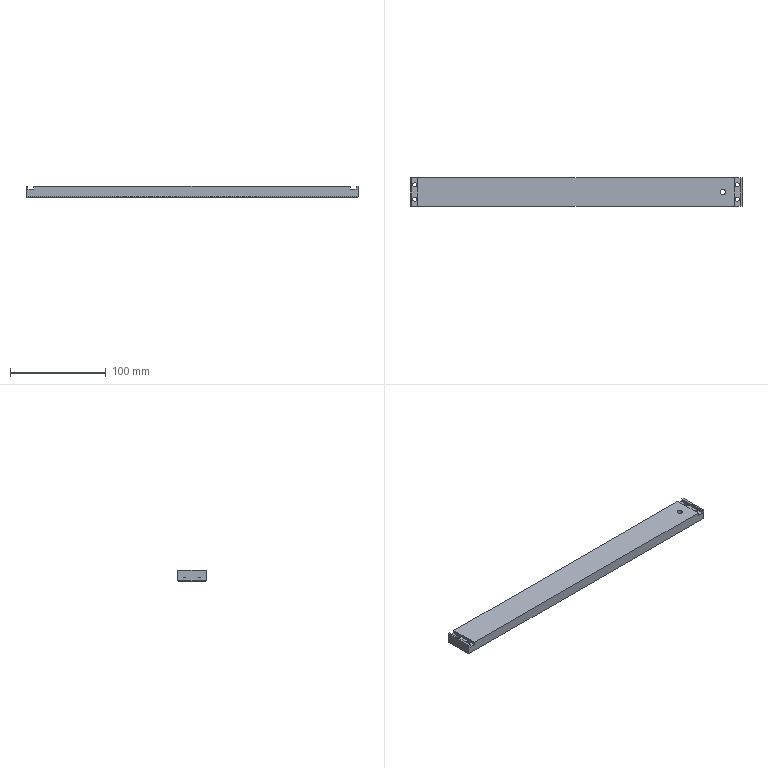Part | NX | 1 solid | 32 faces | box 346 x 30 x 11.5 mm | volume 116609 mm3 | plane 22 | cylinder 9 | cone 1 | commonest cylinder face diameters 4.5 x4 8 x4 5.5 x1
STEP:
#1=CARTESIAN_POINT('',(0.,30.,0.75));
#2=VERTEX_POINT('',#1);
#3=CARTESIAN_POINT('',(0.75,29.25,0.));
#4=VERTEX_POINT('',#3);
#5=CARTESIAN_POINT('',(0.,30.,0.75));
#6=DIRECTION('',(0.5774,-0.5774,-0.5774));
#7=VECTOR('',#6,1000.);
#8=LINE('',#5,#7);
#9=EDGE_CURVE('',#2,#4,#8,.T.);
#10=ORIENTED_EDGE('',*,*,#9,.T.);
#11=CARTESIAN_POINT('',(0.75,0.75,0.));
#12=VERTEX_POINT('',#11);
#13=CARTESIAN_POINT('',(0.75,30.,0.));
#14=DIRECTION('',(0.,1.,0.));
#15=VECTOR('',#14,1000.);
#16=LINE('',#13,#15);
#17=EDGE_CURVE('',#12,#4,#16,.T.);
#18=ORIENTED_EDGE('',*,*,#17,.F.);
#19=CARTESIAN_POINT('',(0.,0.,0.75));
#20=VERTEX_POINT('',#19);
#21=CARTESIAN_POINT('',(0.,0.,0.75));
#22=DIRECTION('',(-0.5774,-0.5774,0.5774));
#23=VECTOR('',#22,1000.);
#24=LINE('',#21,#23);
#25=EDGE_CURVE('',#12,#20,#24,.T.);
#26=ORIENTED_EDGE('',*,*,#25,.T.);
#27=CARTESIAN_POINT('',(0.,0.,0.75));
#28=DIRECTION('',(0.,-1.,0.));
#29=VECTOR('',#28,1000.);
#30=LINE('',#27,#29);
#31=EDGE_CURVE('',#2,#20,#30,.T.);
#32=ORIENTED_EDGE('',*,*,#31,.F.);
#33=EDGE_LOOP('',(#10,#18,#26,#32));
#34=FACE_BOUND('',#33,.T.);
#35=CARTESIAN_POINT('',(0.,0.,0.75));
#36=DIRECTION('',(-0.7071,0.,-0.7071));
#37=DIRECTION('',(0.,1.,0.));
#38=AXIS2_PLACEMENT_3D('',#35,#36,#37);
#39=PLANE('',#38);
#40=ADVANCED_FACE('',(#34),#39,.T.);
#41=CARTESIAN_POINT('',(345.25,0.75,0.));
#42=VERTEX_POINT('',#41);
#43=CARTESIAN_POINT('',(346.,0.,0.75));
#44=VERTEX_POINT('',#43);
#45=CARTESIAN_POINT('',(230.667,115.333,-114.583));
#46=DIRECTION('',(0.5774,-0.5774,0.5774));
#47=VECTOR('',#46,1000.);
#48=LINE('',#45,#47);
#49=EDGE_CURVE('',#42,#44,#48,.T.);
#50=ORIENTED_EDGE('',*,*,#49,.T.);
#51=CARTESIAN_POINT('',(346.,0.,0.75));
#52=DIRECTION('',(1.,0.,0.));
#53=VECTOR('',#52,1000.);
#54=LINE('',#51,#53);
#55=EDGE_CURVE('',#20,#44,#54,.T.);
#56=ORIENTED_EDGE('',*,*,#55,.F.);
#57=ORIENTED_EDGE('',*,*,#25,.F.);
#58=CARTESIAN_POINT('',(0.,0.75,0.));
#59=DIRECTION('',(-1.,0.,0.));
#60=VECTOR('',#59,1000.);
#61=LINE('',#58,#60);
#62=EDGE_CURVE('',#42,#12,#61,.T.);
#63=ORIENTED_EDGE('',*,*,#62,.F.);
#64=EDGE_LOOP('',(#50,#56,#57,#63));
#65=FACE_BOUND('',#64,.T.);
#66=CARTESIAN_POINT('',(0.,0.,0.75));
#67=DIRECTION('',(0.,-0.7071,-0.7071));
#68=DIRECTION('',(-1.,0.,0.));
#69=AXIS2_PLACEMENT_3D('',#66,#67,#68);
#70=PLANE('',#69);
#71=ADVANCED_FACE('',(#65),#70,.T.);
#72=CARTESIAN_POINT('',(346.,30.,0.75));
#73=VERTEX_POINT('',#72);
#74=CARTESIAN_POINT('',(345.25,29.25,0.));
#75=VERTEX_POINT('',#74);
#76=CARTESIAN_POINT('',(336.,20.,-9.25));
#77=DIRECTION('',(-0.5774,-0.5774,-0.5774));
#78=VECTOR('',#77,1000.);
#79=LINE('',#76,#78);
#80=EDGE_CURVE('',#73,#75,#79,.T.);
#81=ORIENTED_EDGE('',*,*,#80,.T.);
#82=CARTESIAN_POINT('',(346.,29.25,0.));
#83=DIRECTION('',(1.,0.,0.));
#84=VECTOR('',#83,1000.);
#85=LINE('',#82,#84);
#86=EDGE_CURVE('',#4,#75,#85,.T.);
#87=ORIENTED_EDGE('',*,*,#86,.F.);
#88=ORIENTED_EDGE('',*,*,#9,.F.);
#89=CARTESIAN_POINT('',(0.,30.,0.75));
#90=DIRECTION('',(-1.,0.,0.));
#91=VECTOR('',#90,1000.);
#92=LINE('',#89,#91);
#93=EDGE_CURVE('',#73,#2,#92,.T.);
#94=ORIENTED_EDGE('',*,*,#93,.F.);
#95=EDGE_LOOP('',(#81,#87,#88,#94));
#96=FACE_BOUND('',#95,.T.);
#97=CARTESIAN_POINT('',(0.,30.,0.75));
#98=DIRECTION('',(0.,0.7071,-0.7071));
#99=DIRECTION('',(1.,0.,0.));
#100=AXIS2_PLACEMENT_3D('',#97,#98,#99);
#101=PLANE('',#100);
#102=ADVANCED_FACE('',(#96),#101,.T.);
#103=ORIENTED_EDGE('',*,*,#49,.F.);
#104=CARTESIAN_POINT('',(345.25,0.,0.));
#105=DIRECTION('',(0.,-1.,0.));
#106=VECTOR('',#105,1000.);
#107=LINE('',#104,#106);
#108=EDGE_CURVE('',#75,#42,#107,.T.);
#109=ORIENTED_EDGE('',*,*,#108,.F.);
#110=ORIENTED_EDGE('',*,*,#80,.F.);
#111=CARTESIAN_POINT('',(346.,30.,0.75));
#112=DIRECTION('',(0.,1.,0.));
#113=VECTOR('',#112,1000.);
#114=LINE('',#111,#113);
#115=EDGE_CURVE('',#44,#73,#114,.T.);
#116=ORIENTED_EDGE('',*,*,#115,.F.);
#117=EDGE_LOOP('',(#103,#109,#110,#116));
#118=FACE_BOUND('',#117,.T.);
#119=CARTESIAN_POINT('',(346.,0.,0.75));
#120=DIRECTION('',(0.7071,0.,-0.7071));
#121=DIRECTION('',(0.,-1.,0.));
#122=AXIS2_PLACEMENT_3D('',#119,#120,#121);
#123=PLANE('',#122);
#124=ADVANCED_FACE('',(#118),#123,.T.);
#125=CARTESIAN_POINT('',(1.,22.5,4.));
#126=VERTEX_POINT('',#125);
#127=CARTESIAN_POINT('',(5.,22.5,4.));
#128=DIRECTION('',(0.,0.,-1.));
#129=DIRECTION('',(-1.,0.,0.));
#130=AXIS2_PLACEMENT_3D('',#127,#128,#129);
#131=CIRCLE('',#130,4.);
#132=EDGE_CURVE('',#126,#126,#131,.T.);
#133=ORIENTED_EDGE('',*,*,#132,.T.);
#134=EDGE_LOOP('',(#133));
#135=FACE_BOUND('',#134,.T.);
#136=CARTESIAN_POINT('',(2.75,22.5,4.));
#137=VERTEX_POINT('',#136);
#138=CARTESIAN_POINT('',(5.,22.5,4.));
#139=DIRECTION('',(0.,0.,-1.));
#140=DIRECTION('',(-1.,0.,0.));
#141=AXIS2_PLACEMENT_3D('',#138,#139,#140);
#142=CIRCLE('',#141,2.25);
#143=EDGE_CURVE('',#137,#137,#142,.T.);
#144=ORIENTED_EDGE('',*,*,#143,.F.);
#145=EDGE_LOOP('',(#144));
#146=FACE_BOUND('',#145,.T.);
#147=CARTESIAN_POINT('',(7.25,22.5,4.));
#148=DIRECTION('',(0.,0.,1.));
#149=DIRECTION('',(1.,0.,0.));
#150=AXIS2_PLACEMENT_3D('',#147,#148,#149);
#151=PLANE('',#150);
#152=ADVANCED_FACE('',(#135,#146),#151,.F.);
#153=CARTESIAN_POINT('',(9.,7.5,4.));
#154=VERTEX_POINT('',#153);
#155=CARTESIAN_POINT('',(5.,7.5,4.));
#156=DIRECTION('',(0.,0.,-1.));
#157=DIRECTION('',(1.,0.,0.));
#158=AXIS2_PLACEMENT_3D('',#155,#156,#157);
#159=CIRCLE('',#158,4.);
#160=EDGE_CURVE('',#154,#154,#159,.T.);
#161=ORIENTED_EDGE('',*,*,#160,.T.);
#162=EDGE_LOOP('',(#161));
#163=FACE_BOUND('',#162,.T.);
#164=CARTESIAN_POINT('',(7.25,7.5,4.));
#165=VERTEX_POINT('',#164);
#166=CARTESIAN_POINT('',(5.,7.5,4.));
#167=DIRECTION('',(0.,0.,-1.));
#168=DIRECTION('',(1.,0.,0.));
#169=AXIS2_PLACEMENT_3D('',#166,#167,#168);
#170=CIRCLE('',#169,2.25);
#171=EDGE_CURVE('',#165,#165,#170,.T.);
#172=ORIENTED_EDGE('',*,*,#171,.F.);
#173=EDGE_LOOP('',(#172));
#174=FACE_BOUND('',#173,.T.);
#175=CARTESIAN_POINT('',(7.25,22.5,4.));
#176=DIRECTION('',(0.,0.,1.));
#177=DIRECTION('',(1.,0.,0.));
#178=AXIS2_PLACEMENT_3D('',#175,#176,#177);
#179=PLANE('',#178);
#180=ADVANCED_FACE('',(#163,#174),#179,.F.);
#181=CARTESIAN_POINT('',(8.,30.,8.5));
#182=VERTEX_POINT('',#181);
#183=CARTESIAN_POINT('',(8.,30.,11.5));
#184=VERTEX_POINT('',#183);
#185=CARTESIAN_POINT('',(8.,30.,11.5));
#186=DIRECTION('',(0.,0.,1.));
#187=VECTOR('',#186,1000.);
#188=LINE('',#185,#187);
#189=EDGE_CURVE('',#182,#184,#188,.T.);
#190=ORIENTED_EDGE('',*,*,#189,.F.);
#191=CARTESIAN_POINT('',(8.,0.,8.5));
#192=VERTEX_POINT('',#191);
#193=CARTESIAN_POINT('',(8.,0.,8.5));
#194=DIRECTION('',(0.,1.,0.));
#195=VECTOR('',#194,1000.);
#196=LINE('',#193,#195);
#197=EDGE_CURVE('',#192,#182,#196,.T.);
#198=ORIENTED_EDGE('',*,*,#197,.F.);
#199=CARTESIAN_POINT('',(8.,0.,11.5));
#200=VERTEX_POINT('',#199);
#201=CARTESIAN_POINT('',(8.,0.,11.5));
#202=DIRECTION('',(0.,0.,1.));
#203=VECTOR('',#202,1000.);
#204=LINE('',#201,#203);
#205=EDGE_CURVE('',#192,#200,#204,.T.);
#206=ORIENTED_EDGE('',*,*,#205,.T.);
#207=CARTESIAN_POINT('',(8.,0.,11.5));
#208=DIRECTION('',(0.,1.,0.));
#209=VECTOR('',#208,1000.);
#210=LINE('',#207,#209);
#211=EDGE_CURVE('',#200,#184,#210,.T.);
#212=ORIENTED_EDGE('',*,*,#211,.T.);
#213=EDGE_LOOP('',(#190,#198,#206,#212));
#214=FACE_BOUND('',#213,.T.);
#215=CARTESIAN_POINT('',(8.,0.,11.5));
#216=DIRECTION('',(-1.,0.,0.));
#217=DIRECTION('',(0.,0.,1.));
#218=AXIS2_PLACEMENT_3D('',#215,#216,#217);
#219=PLANE('',#218);
#220=ADVANCED_FACE('',(#214),#219,.T.);
#221=CARTESIAN_POINT('',(2.,30.,8.5));
#222=VERTEX_POINT('',#221);
#223=CARTESIAN_POINT('',(2.,30.,8.5));
#224=DIRECTION('',(1.,0.,0.));
#225=VECTOR('',#224,1000.);
#226=LINE('',#223,#225);
#227=EDGE_CURVE('',#222,#182,#226,.T.);
#228=ORIENTED_EDGE('',*,*,#227,.F.);
#229=CARTESIAN_POINT('',(2.,0.,8.5));
#230=VERTEX_POINT('',#229);
#231=CARTESIAN_POINT('',(2.,0.,8.5));
#232=DIRECTION('',(0.,1.,0.));
#233=VECTOR('',#232,1000.);
#234=LINE('',#231,#233);
#235=EDGE_CURVE('',#230,#222,#234,.T.);
#236=ORIENTED_EDGE('',*,*,#235,.F.);
#237=CARTESIAN_POINT('',(2.,0.,8.5));
#238=DIRECTION('',(1.,0.,0.));
#239=VECTOR('',#238,1000.);
#240=LINE('',#237,#239);
#241=EDGE_CURVE('',#230,#192,#240,.T.);
#242=ORIENTED_EDGE('',*,*,#241,.T.);
#243=ORIENTED_EDGE('',*,*,#197,.T.);
#244=EDGE_LOOP('',(#228,#236,#242,#243));
#245=FACE_BOUND('',#244,.T.);
#246=CARTESIAN_POINT('',(7.25,7.5,8.5));
#247=VERTEX_POINT('',#246);
#248=CARTESIAN_POINT('',(5.,7.5,8.5));
#249=DIRECTION('',(0.,0.,1.));
#250=DIRECTION('',(1.,0.,0.));
#251=AXIS2_PLACEMENT_3D('',#248,#249,#250);
#252=CIRCLE('',#251,2.25);
#253=EDGE_CURVE('',#247,#247,#252,.T.);
#254=ORIENTED_EDGE('',*,*,#253,.F.);
#255=EDGE_LOOP('',(#254));
#256=FACE_BOUND('',#255,.T.);
#257=CARTESIAN_POINT('',(7.25,22.5,8.5));
#258=VERTEX_POINT('',#257);
#259=CARTESIAN_POINT('',(5.,22.5,8.5));
#260=DIRECTION('',(0.,0.,1.));
#261=DIRECTION('',(1.,0.,0.));
#262=AXIS2_PLACEMENT_3D('',#259,#260,#261);
#263=CIRCLE('',#262,2.25);
#264=EDGE_CURVE('',#258,#258,#263,.T.);
#265=ORIENTED_EDGE('',*,*,#264,.F.);
#266=EDGE_LOOP('',(#265));
#267=FACE_BOUND('',#266,.T.);
#268=CARTESIAN_POINT('',(2.,0.,8.5));
#269=DIRECTION('',(0.,0.,1.));
#270=DIRECTION('',(1.,0.,0.));
#271=AXIS2_PLACEMENT_3D('',#268,#269,#270);
#272=PLANE('',#271);
#273=ADVANCED_FACE('',(#245,#256,#267),#272,.T.);
#274=CARTESIAN_POINT('',(2.,30.,11.5));
#275=VERTEX_POINT('',#274);
#276=CARTESIAN_POINT('',(2.,30.,11.5));
#277=DIRECTION('',(0.,0.,-1.));
#278=VECTOR('',#277,1000.);
#279=LINE('',#276,#278);
#280=EDGE_CURVE('',#275,#222,#279,.T.);
#281=ORIENTED_EDGE('',*,*,#280,.F.);
#282=CARTESIAN_POINT('',(2.,0.,11.5));
#283=VERTEX_POINT('',#282);
#284=CARTESIAN_POINT('',(2.,0.,11.5));
#285=DIRECTION('',(0.,1.,0.));
#286=VECTOR('',#285,1000.);
#287=LINE('',#284,#286);
#288=EDGE_CURVE('',#283,#275,#287,.T.);
#289=ORIENTED_EDGE('',*,*,#288,.F.);
#290=CARTESIAN_POINT('',(2.,0.,11.5));
#291=DIRECTION('',(0.,0.,-1.));
#292=VECTOR('',#291,1000.);
#293=LINE('',#290,#292);
#294=EDGE_CURVE('',#283,#230,#293,.T.);
#295=ORIENTED_EDGE('',*,*,#294,.T.);
#296=ORIENTED_EDGE('',*,*,#235,.T.);
#297=EDGE_LOOP('',(#281,#289,#295,#296));
#298=FACE_BOUND('',#297,.T.);
#299=CARTESIAN_POINT('',(2.,0.,11.5));
#300=DIRECTION('',(1.,0.,0.));
#301=DIRECTION('',(0.,0.,-1.));
#302=AXIS2_PLACEMENT_3D('',#299,#300,#301);
#303=PLANE('',#302);
#304=ADVANCED_FACE('',(#298),#303,.T.);
#305=CARTESIAN_POINT('',(345.,22.5,4.));
#306=VERTEX_POINT('',#305);
#307=CARTESIAN_POINT('',(341.,22.5,4.));
#308=DIRECTION('',(0.,0.,-1.));
#309=DIRECTION('',(1.,0.,0.));
#310=AXIS2_PLACEMENT_3D('',#307,#308,#309);
#311=CIRCLE('',#310,4.);
#312=EDGE_CURVE('',#306,#306,#311,.T.);
#313=ORIENTED_EDGE('',*,*,#312,.T.);
#314=EDGE_LOOP('',(#313));
#315=FACE_BOUND('',#314,.T.);
#316=CARTESIAN_POINT('',(343.25,22.5,4.));
#317=VERTEX_POINT('',#316);
#318=CARTESIAN_POINT('',(341.,22.5,4.));
#319=DIRECTION('',(0.,0.,-1.));
#320=DIRECTION('',(1.,0.,0.));
#321=AXIS2_PLACEMENT_3D('',#318,#319,#320);
#322=CIRCLE('',#321,2.25);
#323=EDGE_CURVE('',#317,#317,#322,.T.);
#324=ORIENTED_EDGE('',*,*,#323,.F.);
#325=EDGE_LOOP('',(#324));
#326=FACE_BOUND('',#325,.T.);
#327=CARTESIAN_POINT('',(7.25,22.5,4.));
#328=DIRECTION('',(0.,0.,1.));
#329=DIRECTION('',(1.,0.,0.));
#330=AXIS2_PLACEMENT_3D('',#327,#328,#329);
#331=PLANE('',#330);
#332=ADVANCED_FACE('',(#315,#326),#331,.F.);
#333=CARTESIAN_POINT('',(345.,7.5,4.));
#334=VERTEX_POINT('',#333);
#335=CARTESIAN_POINT('',(341.,7.5,4.));
#336=DIRECTION('',(0.,0.,-1.));
#337=DIRECTION('',(1.,0.,0.));
#338=AXIS2_PLACEMENT_3D('',#335,#336,#337);
#339=CIRCLE('',#338,4.);
#340=EDGE_CURVE('',#334,#334,#339,.T.);
#341=ORIENTED_EDGE('',*,*,#340,.T.);
#342=EDGE_LOOP('',(#341));
#343=FACE_BOUND('',#342,.T.);
#344=CARTESIAN_POINT('',(343.25,7.5,4.));
#345=VERTEX_POINT('',#344);
#346=CARTESIAN_POINT('',(341.,7.5,4.));
#347=DIRECTION('',(0.,0.,-1.));
#348=DIRECTION('',(1.,0.,0.));
#349=AXIS2_PLACEMENT_3D('',#346,#347,#348);
#350=CIRCLE('',#349,2.25);
#351=EDGE_CURVE('',#345,#345,#350,.T.);
#352=ORIENTED_EDGE('',*,*,#351,.F.);
#353=EDGE_LOOP('',(#352));
#354=FACE_BOUND('',#353,.T.);
#355=CARTESIAN_POINT('',(7.25,22.5,4.));
#356=DIRECTION('',(0.,0.,1.));
#357=DIRECTION('',(1.,0.,0.));
#358=AXIS2_PLACEMENT_3D('',#355,#356,#357);
#359=PLANE('',#358);
#360=ADVANCED_FACE('',(#343,#354),#359,.F.);
#361=CARTESIAN_POINT('',(344.,30.,8.5));
#362=VERTEX_POINT('',#361);
#363=CARTESIAN_POINT('',(338.,30.,8.5));
#364=VERTEX_POINT('',#363);
#365=CARTESIAN_POINT('',(2.,30.,8.5));
#366=DIRECTION('',(-1.,0.,0.));
#367=VECTOR('',#366,1000.);
#368=LINE('',#365,#367);
#369=EDGE_CURVE('',#362,#364,#368,.T.);
#370=ORIENTED_EDGE('',*,*,#369,.T.);
#371=CARTESIAN_POINT('',(338.,0.,8.5));
#372=VERTEX_POINT('',#371);
#373=CARTESIAN_POINT('',(338.,0.,8.5));
#374=DIRECTION('',(0.,1.,0.));
#375=VECTOR('',#374,1000.);
#376=LINE('',#373,#375);
#377=EDGE_CURVE('',#372,#364,#376,.T.);
#378=ORIENTED_EDGE('',*,*,#377,.F.);
#379=CARTESIAN_POINT('',(344.,0.,8.5));
#380=VERTEX_POINT('',#379);
#381=CARTESIAN_POINT('',(0.,0.,8.5));
#382=DIRECTION('',(-1.,0.,0.));
#383=VECTOR('',#382,1000.);
#384=LINE('',#381,#383);
#385=EDGE_CURVE('',#380,#372,#384,.T.);
#386=ORIENTED_EDGE('',*,*,#385,.F.);
#387=CARTESIAN_POINT('',(344.,0.,8.5));
#388=DIRECTION('',(0.,1.,0.));
#389=VECTOR('',#388,1000.);
#390=LINE('',#387,#389);
#391=EDGE_CURVE('',#380,#362,#390,.T.);
#392=ORIENTED_EDGE('',*,*,#391,.T.);
#393=EDGE_LOOP('',(#370,#378,#386,#392));
#394=FACE_BOUND('',#393,.T.);
#395=CARTESIAN_POINT('',(343.25,7.5,8.5));
#396=VERTEX_POINT('',#395);
#397=CARTESIAN_POINT('',(341.,7.5,8.5));
#398=DIRECTION('',(0.,0.,-1.));
#399=DIRECTION('',(1.,0.,0.));
#400=AXIS2_PLACEMENT_3D('',#397,#398,#399);
#401=CIRCLE('',#400,2.25);
#402=EDGE_CURVE('',#396,#396,#401,.T.);
#403=ORIENTED_EDGE('',*,*,#402,.T.);
#404=EDGE_LOOP('',(#403));
#405=FACE_BOUND('',#404,.T.);
#406=CARTESIAN_POINT('',(343.25,22.5,8.5));
#407=VERTEX_POINT('',#406);
#408=CARTESIAN_POINT('',(341.,22.5,8.5));
#409=DIRECTION('',(0.,0.,-1.));
#410=DIRECTION('',(1.,0.,0.));
#411=AXIS2_PLACEMENT_3D('',#408,#409,#410);
#412=CIRCLE('',#411,2.25);
#413=EDGE_CURVE('',#407,#407,#412,.T.);
#414=ORIENTED_EDGE('',*,*,#413,.T.);
#415=EDGE_LOOP('',(#414));
#416=FACE_BOUND('',#415,.T.);
#417=CARTESIAN_POINT('',(2.,0.,8.5));
#418=DIRECTION('',(0.,0.,1.));
#419=DIRECTION('',(1.,0.,0.));
#420=AXIS2_PLACEMENT_3D('',#417,#418,#419);
#421=PLANE('',#420);
#422=ADVANCED_FACE('',(#394,#405,#416),#421,.T.);
#423=CARTESIAN_POINT('',(338.,30.,11.5));
#424=VERTEX_POINT('',#423);
#425=CARTESIAN_POINT('',(338.,30.,11.5));
#426=DIRECTION('',(0.,0.,1.));
#427=VECTOR('',#426,1000.);
#428=LINE('',#425,#427);
#429=EDGE_CURVE('',#364,#424,#428,.T.);
#430=ORIENTED_EDGE('',*,*,#429,.T.);
#431=CARTESIAN_POINT('',(338.,0.,11.5));
#432=VERTEX_POINT('',#431);
#433=CARTESIAN_POINT('',(338.,0.,11.5));
#434=DIRECTION('',(0.,1.,0.));
#435=VECTOR('',#434,1000.);
#436=LINE('',#433,#435);
#437=EDGE_CURVE('',#432,#424,#436,.T.);
#438=ORIENTED_EDGE('',*,*,#437,.F.);
#439=CARTESIAN_POINT('',(338.,0.,11.5));
#440=DIRECTION('',(0.,0.,1.));
#441=VECTOR('',#440,1000.);
#442=LINE('',#439,#441);
#443=EDGE_CURVE('',#372,#432,#442,.T.);
#444=ORIENTED_EDGE('',*,*,#443,.F.);
#445=ORIENTED_EDGE('',*,*,#377,.T.);
#446=EDGE_LOOP('',(#430,#438,#444,#445));
#447=FACE_BOUND('',#446,.T.);
#448=CARTESIAN_POINT('',(338.,0.,11.5));
#449=DIRECTION('',(-1.,0.,0.));
#450=DIRECTION('',(0.,0.,1.));
#451=AXIS2_PLACEMENT_3D('',#448,#449,#450);
#452=PLANE('',#451);
#453=ADVANCED_FACE('',(#447),#452,.F.);
#454=CARTESIAN_POINT('',(344.,30.,11.5));
#455=VERTEX_POINT('',#454);
#456=CARTESIAN_POINT('',(344.,30.,11.5));
#457=DIRECTION('',(0.,0.,-1.));
#458=VECTOR('',#457,1000.);
#459=LINE('',#456,#458);
#460=EDGE_CURVE('',#455,#362,#459,.T.);
#461=ORIENTED_EDGE('',*,*,#460,.T.);
#462=ORIENTED_EDGE('',*,*,#391,.F.);
#463=CARTESIAN_POINT('',(344.,0.,11.5));
#464=VERTEX_POINT('',#463);
#465=CARTESIAN_POINT('',(344.,0.,11.5));
#466=DIRECTION('',(0.,0.,-1.));
#467=VECTOR('',#466,1000.);
#468=LINE('',#465,#467);
#469=EDGE_CURVE('',#464,#380,#468,.T.);
#470=ORIENTED_EDGE('',*,*,#469,.F.);
#471=CARTESIAN_POINT('',(344.,0.,11.5));
#472=DIRECTION('',(0.,1.,0.));
#473=VECTOR('',#472,1000.);
#474=LINE('',#471,#473);
#475=EDGE_CURVE('',#464,#455,#474,.T.);
#476=ORIENTED_EDGE('',*,*,#475,.T.);
#477=EDGE_LOOP('',(#461,#462,#470,#476));
#478=FACE_BOUND('',#477,.T.);
#479=CARTESIAN_POINT('',(344.,0.,11.5));
#480=DIRECTION('',(1.,0.,0.));
#481=DIRECTION('',(0.,0.,-1.));
#482=AXIS2_PLACEMENT_3D('',#479,#480,#481);
#483=PLANE('',#482);
#484=ADVANCED_FACE('',(#478),#483,.F.);
#485=CARTESIAN_POINT('',(337.,7.5,0.));
#486=VERTEX_POINT('',#485);
#487=CARTESIAN_POINT('',(341.,7.5,0.));
#488=DIRECTION('',(0.,0.,-1.));
#489=DIRECTION('',(-1.,0.,0.));
#490=AXIS2_PLACEMENT_3D('',#487,#488,#489);
#491=CIRCLE('',#490,4.);
#492=EDGE_CURVE('',#486,#486,#491,.T.);
#493=ORIENTED_EDGE('',*,*,#492,.F.);
#494=EDGE_LOOP('',(#493));
#495=FACE_BOUND('',#494,.T.);
#496=CARTESIAN_POINT('',(337.,22.5,0.));
#497=VERTEX_POINT('',#496);
#498=CARTESIAN_POINT('',(341.,22.5,0.));
#499=DIRECTION('',(0.,0.,-1.));
#500=DIRECTION('',(-1.,0.,0.));
#501=AXIS2_PLACEMENT_3D('',#498,#499,#500);
#502=CIRCLE('',#501,4.);
#503=EDGE_CURVE('',#497,#497,#502,.T.);
#504=ORIENTED_EDGE('',*,*,#503,.F.);
#505=EDGE_LOOP('',(#504));
#506=FACE_BOUND('',#505,.T.);
#507=CARTESIAN_POINT('',(1.,7.5,0.));
#508=VERTEX_POINT('',#507);
#509=CARTESIAN_POINT('',(5.,7.5,0.));
#510=DIRECTION('',(0.,0.,-1.));
#511=DIRECTION('',(-1.,0.,0.));
#512=AXIS2_PLACEMENT_3D('',#509,#510,#511);
#513=CIRCLE('',#512,4.);
#514=EDGE_CURVE('',#508,#508,#513,.T.);
#515=ORIENTED_EDGE('',*,*,#514,.F.);
#516=EDGE_LOOP('',(#515));
#517=FACE_BOUND('',#516,.T.);
#518=CARTESIAN_POINT('',(1.,22.5,0.));
#519=VERTEX_POINT('',#518);
#520=CARTESIAN_POINT('',(5.,22.5,0.));
#521=DIRECTION('',(0.,0.,-1.));
#522=DIRECTION('',(-1.,0.,0.));
#523=AXIS2_PLACEMENT_3D('',#520,#521,#522);
#524=CIRCLE('',#523,4.);
#525=EDGE_CURVE('',#519,#519,#524,.T.);
#526=ORIENTED_EDGE('',*,*,#525,.F.);
#527=EDGE_LOOP('',(#526));
#528=FACE_BOUND('',#527,.T.);
#529=CARTESIAN_POINT('',(320.25,15.,0.));
#530=VERTEX_POINT('',#529);
#531=CARTESIAN_POINT('',(326.,15.,0.));
#532=DIRECTION('',(0.,0.,1.));
#533=DIRECTION('',(-1.,0.,0.));
#534=AXIS2_PLACEMENT_3D('',#531,#532,#533);
#535=CIRCLE('',#534,5.75);
#536=EDGE_CURVE('',#530,#530,#535,.T.);
#537=ORIENTED_EDGE('',*,*,#536,.T.);
#538=EDGE_LOOP('',(#537));
#539=FACE_BOUND('',#538,.T.);
#540=ORIENTED_EDGE('',*,*,#62,.T.);
#541=ORIENTED_EDGE('',*,*,#17,.T.);
#542=ORIENTED_EDGE('',*,*,#86,.T.);
#543=ORIENTED_EDGE('',*,*,#108,.T.);
#544=EDGE_LOOP('',(#540,#541,#542,#543));
#545=FACE_BOUND('',#544,.T.);
#546=CARTESIAN_POINT('',(0.,0.,0.));
#547=DIRECTION('',(0.,0.,-1.));
#548=DIRECTION('',(-1.,0.,0.));
#549=AXIS2_PLACEMENT_3D('',#546,#547,#548);
#550=PLANE('',#549);
#551=ADVANCED_FACE('',(#495,#506,#517,#528,#539,#545),#550,.T.);
#552=CARTESIAN_POINT('',(346.,0.,11.5));
#553=VERTEX_POINT('',#552);
#554=CARTESIAN_POINT('',(346.,0.,11.5));
#555=DIRECTION('',(0.,0.,-1.));
#556=VECTOR('',#555,1000.);
#557=LINE('',#554,#556);
#558=EDGE_CURVE('',#553,#44,#557,.T.);
#559=ORIENTED_EDGE('',*,*,#558,.T.);
#560=ORIENTED_EDGE('',*,*,#115,.T.);
#561=CARTESIAN_POINT('',(346.,30.,11.5));
#562=VERTEX_POINT('',#561);
#563=CARTESIAN_POINT('',(346.,30.,11.5));
#564=DIRECTION('',(0.,0.,-1.));
#565=VECTOR('',#564,1000.);
#566=LINE('',#563,#565);
#567=EDGE_CURVE('',#562,#73,#566,.T.);
#568=ORIENTED_EDGE('',*,*,#567,.F.);
#569=CARTESIAN_POINT('',(346.,0.,11.5));
#570=DIRECTION('',(0.,1.,0.));
#571=VECTOR('',#570,1000.);
#572=LINE('',#569,#571);
#573=EDGE_CURVE('',#553,#562,#572,.T.);
#574=ORIENTED_EDGE('',*,*,#573,.F.);
#575=EDGE_LOOP('',(#559,#560,#568,#574));
#576=FACE_BOUND('',#575,.T.);
#577=CARTESIAN_POINT('',(346.,0.,11.5));
#578=DIRECTION('',(-1.,0.,0.));
#579=DIRECTION('',(0.,0.,1.));
#580=AXIS2_PLACEMENT_3D('',#577,#578,#579);
#581=PLANE('',#580);
#582=ADVANCED_FACE('',(#576),#581,.F.);
#583=CARTESIAN_POINT('',(0.,30.,11.5));
#584=VERTEX_POINT('',#583);
#585=CARTESIAN_POINT('',(0.,30.,11.5));
#586=DIRECTION('',(0.,0.,-1.));
#587=VECTOR('',#586,1000.);
#588=LINE('',#585,#587);
#589=EDGE_CURVE('',#584,#2,#588,.T.);
#590=ORIENTED_EDGE('',*,*,#589,.T.);
#591=ORIENTED_EDGE('',*,*,#31,.T.);
#592=CARTESIAN_POINT('',(0.,0.,11.5));
#593=VERTEX_POINT('',#592);
#594=CARTESIAN_POINT('',(0.,0.,11.5));
#595=DIRECTION('',(0.,0.,-1.));
#596=VECTOR('',#595,1000.);
#597=LINE('',#594,#596);
#598=EDGE_CURVE('',#593,#20,#597,.T.);
#599=ORIENTED_EDGE('',*,*,#598,.F.);
#600=CARTESIAN_POINT('',(0.,0.,11.5));
#601=DIRECTION('',(0.,-1.,0.));
#602=VECTOR('',#601,1000.);
#603=LINE('',#600,#602);
#604=EDGE_CURVE('',#584,#593,#603,.T.);
#605=ORIENTED_EDGE('',*,*,#604,.F.);
#606=EDGE_LOOP('',(#590,#591,#599,#605));
#607=FACE_BOUND('',#606,.T.);
#608=CARTESIAN_POINT('',(0.,0.,11.5));
#609=DIRECTION('',(1.,0.,0.));
#610=DIRECTION('',(0.,0.,-1.));
#611=AXIS2_PLACEMENT_3D('',#608,#609,#610);
#612=PLANE('',#611);
#613=ADVANCED_FACE('',(#607),#612,.F.);
#614=CARTESIAN_POINT('',(0.,30.,11.5));
#615=DIRECTION('',(-1.,0.,0.));
#616=VECTOR('',#615,1000.);
#617=LINE('',#614,#616);
#618=EDGE_CURVE('',#562,#455,#617,.T.);
#619=ORIENTED_EDGE('',*,*,#618,.T.);
#620=ORIENTED_EDGE('',*,*,#475,.F.);
#621=CARTESIAN_POINT('',(0.,0.,11.5));
#622=DIRECTION('',(1.,0.,0.));
#623=VECTOR('',#622,1000.);
#624=LINE('',#621,#623);
#625=EDGE_CURVE('',#464,#553,#624,.T.);
#626=ORIENTED_EDGE('',*,*,#625,.T.);
#627=ORIENTED_EDGE('',*,*,#573,.T.);
#628=EDGE_LOOP('',(#619,#620,#626,#627));
#629=FACE_BOUND('',#628,.T.);
#630=CARTESIAN_POINT('',(0.,0.,11.5));
#631=DIRECTION('',(0.,0.,-1.));
#632=DIRECTION('',(-1.,0.,0.));
#633=AXIS2_PLACEMENT_3D('',#630,#631,#632);
#634=PLANE('',#633);
#635=ADVANCED_FACE('',(#629),#634,.F.);
#636=ORIENTED_EDGE('',*,*,#211,.F.);
#637=CARTESIAN_POINT('',(0.,0.,11.5));
#638=DIRECTION('',(1.,0.,0.));
#639=VECTOR('',#638,1000.);
#640=LINE('',#637,#639);
#641=EDGE_CURVE('',#200,#432,#640,.T.);
#642=ORIENTED_EDGE('',*,*,#641,.T.);
#643=ORIENTED_EDGE('',*,*,#437,.T.);
#644=CARTESIAN_POINT('',(0.,30.,11.5));
#645=DIRECTION('',(-1.,0.,0.));
#646=VECTOR('',#645,1000.);
#647=LINE('',#644,#646);
#648=EDGE_CURVE('',#424,#184,#647,.T.);
#649=ORIENTED_EDGE('',*,*,#648,.T.);
#650=EDGE_LOOP('',(#636,#642,#643,#649));
#651=FACE_BOUND('',#650,.T.);
#652=CARTESIAN_POINT('',(323.25,15.,11.5));
#653=VERTEX_POINT('',#652);
#654=CARTESIAN_POINT('',(326.,15.,11.5));
#655=DIRECTION('',(0.,0.,-1.));
#656=DIRECTION('',(-1.,0.,0.));
#657=AXIS2_PLACEMENT_3D('',#654,#655,#656);
#658=CIRCLE('',#657,2.75);
#659=EDGE_CURVE('',#653,#653,#658,.T.);
#660=ORIENTED_EDGE('',*,*,#659,.T.);
#661=EDGE_LOOP('',(#660));
#662=FACE_BOUND('',#661,.T.);
#663=CARTESIAN_POINT('',(0.,0.,11.5));
#664=DIRECTION('',(0.,0.,-1.));
#665=DIRECTION('',(-1.,0.,0.));
#666=AXIS2_PLACEMENT_3D('',#663,#664,#665);
#667=PLANE('',#666);
#668=ADVANCED_FACE('',(#651,#662),#667,.F.);
#669=ORIENTED_EDGE('',*,*,#288,.T.);
#670=CARTESIAN_POINT('',(0.,30.,11.5));
#671=DIRECTION('',(-1.,0.,0.));
#672=VECTOR('',#671,1000.);
#673=LINE('',#670,#672);
#674=EDGE_CURVE('',#275,#584,#673,.T.);
#675=ORIENTED_EDGE('',*,*,#674,.T.);
#676=ORIENTED_EDGE('',*,*,#604,.T.);
#677=CARTESIAN_POINT('',(0.,0.,11.5));
#678=DIRECTION('',(1.,0.,0.));
#679=VECTOR('',#678,1000.);
#680=LINE('',#677,#679);
#681=EDGE_CURVE('',#593,#283,#680,.T.);
#682=ORIENTED_EDGE('',*,*,#681,.T.);
#683=EDGE_LOOP('',(#669,#675,#676,#682));
#684=FACE_BOUND('',#683,.T.);
#685=CARTESIAN_POINT('',(0.,0.,11.5));
#686=DIRECTION('',(0.,0.,-1.));
#687=DIRECTION('',(-1.,0.,0.));
#688=AXIS2_PLACEMENT_3D('',#685,#686,#687);
#689=PLANE('',#688);
#690=ADVANCED_FACE('',(#684),#689,.F.);
#691=ORIENTED_EDGE('',*,*,#567,.T.);
#692=ORIENTED_EDGE('',*,*,#93,.T.);
#693=ORIENTED_EDGE('',*,*,#589,.F.);
#694=ORIENTED_EDGE('',*,*,#674,.F.);
#695=ORIENTED_EDGE('',*,*,#280,.T.);
#696=ORIENTED_EDGE('',*,*,#227,.T.);
#697=ORIENTED_EDGE('',*,*,#189,.T.);
#698=ORIENTED_EDGE('',*,*,#648,.F.);
#699=ORIENTED_EDGE('',*,*,#429,.F.);
#700=ORIENTED_EDGE('',*,*,#369,.F.);
#701=ORIENTED_EDGE('',*,*,#460,.F.);
#702=ORIENTED_EDGE('',*,*,#618,.F.);
#703=EDGE_LOOP('',(#691,#692,#693,#694,#695,#696,#697,#698,#699,#700,#701,#702));
#704=FACE_BOUND('',#703,.T.);
#705=CARTESIAN_POINT('',(0.,30.,11.5));
#706=DIRECTION('',(0.,-1.,0.));
#707=DIRECTION('',(0.,0.,-1.));
#708=AXIS2_PLACEMENT_3D('',#705,#706,#707);
#709=PLANE('',#708);
#710=ADVANCED_FACE('',(#704),#709,.F.);
#711=ORIENTED_EDGE('',*,*,#598,.T.);
#712=ORIENTED_EDGE('',*,*,#55,.T.);
#713=ORIENTED_EDGE('',*,*,#558,.F.);
#714=ORIENTED_EDGE('',*,*,#625,.F.);
#715=ORIENTED_EDGE('',*,*,#469,.T.);
#716=ORIENTED_EDGE('',*,*,#385,.T.);
#717=ORIENTED_EDGE('',*,*,#443,.T.);
#718=ORIENTED_EDGE('',*,*,#641,.F.);
#719=ORIENTED_EDGE('',*,*,#205,.F.);
#720=ORIENTED_EDGE('',*,*,#241,.F.);
#721=ORIENTED_EDGE('',*,*,#294,.F.);
#722=ORIENTED_EDGE('',*,*,#681,.F.);
#723=EDGE_LOOP('',(#711,#712,#713,#714,#715,#716,#717,#718,#719,#720,#721,#722));
#724=FACE_BOUND('',#723,.T.);
#725=CARTESIAN_POINT('',(0.,0.,11.5));
#726=DIRECTION('',(0.,1.,0.));
#727=DIRECTION('',(0.,0.,1.));
#728=AXIS2_PLACEMENT_3D('',#725,#726,#727);
#729=PLANE('',#728);
#730=ADVANCED_FACE('',(#724),#729,.F.);
#731=ORIENTED_EDGE('',*,*,#351,.T.);
#732=EDGE_LOOP('',(#731));
#733=FACE_BOUND('',#732,.T.);
#734=ORIENTED_EDGE('',*,*,#402,.F.);
#735=EDGE_LOOP('',(#734));
#736=FACE_BOUND('',#735,.T.);
#737=CARTESIAN_POINT('',(341.,7.5,0.));
#738=DIRECTION('',(0.,0.,-1.));
#739=DIRECTION('',(-1.,0.,0.));
#740=AXIS2_PLACEMENT_3D('',#737,#738,#739);
#741=CYLINDRICAL_SURFACE('',#740,2.25);
#742=ADVANCED_FACE('',(#733,#736),#741,.F.);
#743=ORIENTED_EDGE('',*,*,#492,.T.);
#744=EDGE_LOOP('',(#743));
#745=FACE_BOUND('',#744,.T.);
#746=ORIENTED_EDGE('',*,*,#340,.F.);
#747=EDGE_LOOP('',(#746));
#748=FACE_BOUND('',#747,.T.);
#749=CARTESIAN_POINT('',(341.,7.5,0.));
#750=DIRECTION('',(0.,0.,-1.));
#751=DIRECTION('',(-1.,0.,0.));
#752=AXIS2_PLACEMENT_3D('',#749,#750,#751);
#753=CYLINDRICAL_SURFACE('',#752,4.);
#754=ADVANCED_FACE('',(#745,#748),#753,.F.);
#755=ORIENTED_EDGE('',*,*,#323,.T.);
#756=EDGE_LOOP('',(#755));
#757=FACE_BOUND('',#756,.T.);
#758=ORIENTED_EDGE('',*,*,#413,.F.);
#759=EDGE_LOOP('',(#758));
#760=FACE_BOUND('',#759,.T.);
#761=CARTESIAN_POINT('',(341.,22.5,0.));
#762=DIRECTION('',(0.,0.,-1.));
#763=DIRECTION('',(-1.,0.,0.));
#764=AXIS2_PLACEMENT_3D('',#761,#762,#763);
#765=CYLINDRICAL_SURFACE('',#764,2.25);
#766=ADVANCED_FACE('',(#757,#760),#765,.F.);
#767=ORIENTED_EDGE('',*,*,#503,.T.);
#768=EDGE_LOOP('',(#767));
#769=FACE_BOUND('',#768,.T.);
#770=ORIENTED_EDGE('',*,*,#312,.F.);
#771=EDGE_LOOP('',(#770));
#772=FACE_BOUND('',#771,.T.);
#773=CARTESIAN_POINT('',(341.,22.5,0.));
#774=DIRECTION('',(0.,0.,-1.));
#775=DIRECTION('',(-1.,0.,0.));
#776=AXIS2_PLACEMENT_3D('',#773,#774,#775);
#777=CYLINDRICAL_SURFACE('',#776,4.);
#778=ADVANCED_FACE('',(#769,#772),#777,.F.);
#779=ORIENTED_EDGE('',*,*,#171,.T.);
#780=EDGE_LOOP('',(#779));
#781=FACE_BOUND('',#780,.T.);
#782=ORIENTED_EDGE('',*,*,#253,.T.);
#783=EDGE_LOOP('',(#782));
#784=FACE_BOUND('',#783,.T.);
#785=CARTESIAN_POINT('',(5.,7.5,0.));
#786=DIRECTION('',(0.,0.,-1.));
#787=DIRECTION('',(-1.,0.,0.));
#788=AXIS2_PLACEMENT_3D('',#785,#786,#787);
#789=CYLINDRICAL_SURFACE('',#788,2.25);
#790=ADVANCED_FACE('',(#781,#784),#789,.F.);
#791=ORIENTED_EDGE('',*,*,#514,.T.);
#792=EDGE_LOOP('',(#791));
#793=FACE_BOUND('',#792,.T.);
#794=ORIENTED_EDGE('',*,*,#160,.F.);
#795=EDGE_LOOP('',(#794));
#796=FACE_BOUND('',#795,.T.);
#797=CARTESIAN_POINT('',(5.,7.5,0.));
#798=DIRECTION('',(0.,0.,-1.));
#799=DIRECTION('',(-1.,0.,0.));
#800=AXIS2_PLACEMENT_3D('',#797,#798,#799);
#801=CYLINDRICAL_SURFACE('',#800,4.);
#802=ADVANCED_FACE('',(#793,#796),#801,.F.);
#803=ORIENTED_EDGE('',*,*,#143,.T.);
#804=EDGE_LOOP('',(#803));
#805=FACE_BOUND('',#804,.T.);
#806=ORIENTED_EDGE('',*,*,#264,.T.);
#807=EDGE_LOOP('',(#806));
#808=FACE_BOUND('',#807,.T.);
#809=CARTESIAN_POINT('',(5.,22.5,0.));
#810=DIRECTION('',(0.,0.,-1.));
#811=DIRECTION('',(-1.,0.,0.));
#812=AXIS2_PLACEMENT_3D('',#809,#810,#811);
#813=CYLINDRICAL_SURFACE('',#812,2.25);
#814=ADVANCED_FACE('',(#805,#808),#813,.F.);
#815=ORIENTED_EDGE('',*,*,#525,.T.);
#816=EDGE_LOOP('',(#815));
#817=FACE_BOUND('',#816,.T.);
#818=ORIENTED_EDGE('',*,*,#132,.F.);
#819=EDGE_LOOP('',(#818));
#820=FACE_BOUND('',#819,.T.);
#821=CARTESIAN_POINT('',(5.,22.5,0.));
#822=DIRECTION('',(0.,0.,-1.));
#823=DIRECTION('',(-1.,0.,0.));
#824=AXIS2_PLACEMENT_3D('',#821,#822,#823);
#825=CYLINDRICAL_SURFACE('',#824,4.);
#826=ADVANCED_FACE('',(#817,#820),#825,.F.);
#827=CARTESIAN_POINT('',(323.25,15.,3.));
#828=VERTEX_POINT('',#827);
#829=CARTESIAN_POINT('',(326.,15.,3.));
#830=DIRECTION('',(0.,0.,-1.));
#831=DIRECTION('',(-1.,0.,0.));
#832=AXIS2_PLACEMENT_3D('',#829,#830,#831);
#833=CIRCLE('',#832,2.75);
#834=EDGE_CURVE('',#828,#828,#833,.T.);
#835=ORIENTED_EDGE('',*,*,#834,.T.);
#836=EDGE_LOOP('',(#835));
#837=FACE_BOUND('',#836,.T.);
#838=ORIENTED_EDGE('',*,*,#659,.F.);
#839=EDGE_LOOP('',(#838));
#840=FACE_BOUND('',#839,.T.);
#841=CARTESIAN_POINT('',(326.,15.,11.5));
#842=DIRECTION('',(0.,0.,-1.));
#843=DIRECTION('',(-1.,0.,0.));
#844=AXIS2_PLACEMENT_3D('',#841,#842,#843);
#845=CYLINDRICAL_SURFACE('',#844,2.75);
#846=ADVANCED_FACE('',(#837,#840),#845,.F.);
#847=ORIENTED_EDGE('',*,*,#536,.F.);
#848=EDGE_LOOP('',(#847));
#849=FACE_BOUND('',#848,.T.);
#850=ORIENTED_EDGE('',*,*,#834,.F.);
#851=EDGE_LOOP('',(#850));
#852=FACE_BOUND('',#851,.T.);
#853=CARTESIAN_POINT('',(326.,15.,3.));
#854=DIRECTION('',(0.,0.,-1.));
#855=DIRECTION('',(-1.,0.,0.));
#856=AXIS2_PLACEMENT_3D('',#853,#854,#855);
#857=CONICAL_SURFACE('',#856,2.75,0.7854);
#858=ADVANCED_FACE('',(#849,#852),#857,.F.);
#859=CLOSED_SHELL('',(#40,#71,#102,#124,#152,#180,#220,#273,#304,#332,#360,#422,#453,#484,#551,#582,#613,#635,#668,#690,#710,#730,#742,#754,#766,#778,#790,#802,#814,#826,#846,#858));
#860=MANIFOLD_SOLID_BREP('',#859);
#861=(LENGTH_UNIT()NAMED_UNIT(*)SI_UNIT(.MILLI.,.METRE.));
#862=UNCERTAINTY_MEASURE_WITH_UNIT(LENGTH_MEASURE(0.00001),#861,'','');
#863=(NAMED_UNIT(*)PLANE_ANGLE_UNIT()SI_UNIT($,.RADIAN.));
#864=(NAMED_UNIT(*)SI_UNIT($,.STERADIAN.)SOLID_ANGLE_UNIT());
#865=(GEOMETRIC_REPRESENTATION_CONTEXT(3)GLOBAL_UNCERTAINTY_ASSIGNED_CONTEXT((#862))GLOBAL_UNIT_ASSIGNED_CONTEXT((#861,#863,#864))REPRESENTATION_CONTEXT('',''));
#866=ADVANCED_BREP_SHAPE_REPRESENTATION('',(#860),#865);